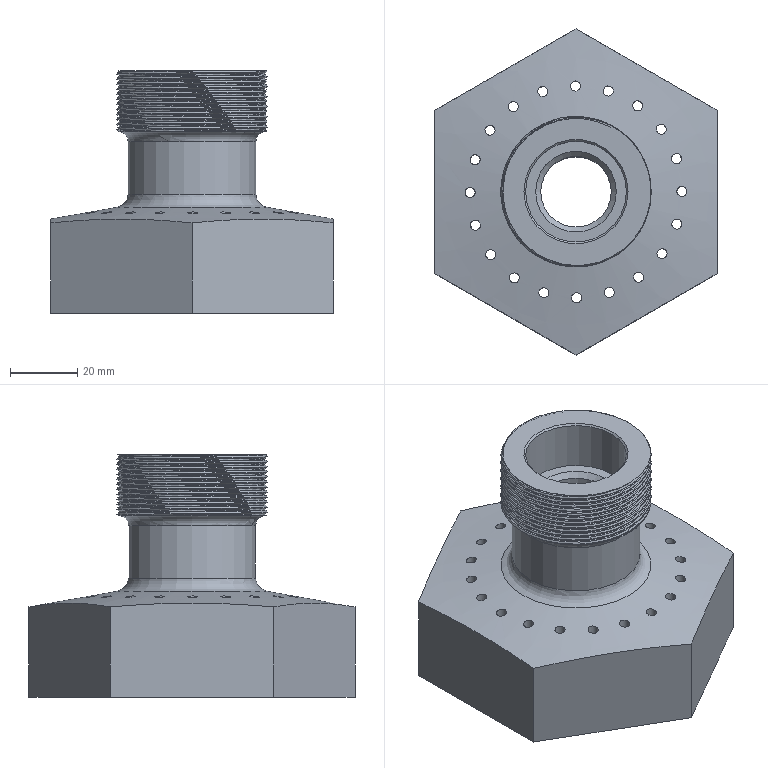Part | NX | features CYLINDER 5, DATUM_CSYS 5, SKETCH 4, BLEND 3, CHAMFER 2, EXTRUDE 2, HOLE PACKAGE 2, SIMPLE HOLE 2, SWP104 2, THREADS 2, REPLACE_FACE 1, SYMBOLIC_THREAD 1 | 1 solid | 56 faces | box 84 x 96.995 x 72 mm | volume 147613 mm3 | cylinder 29 | plane 14 | spline 6 | cone 4 | torus 3 | commonest cylinder face diameters 3 x20 72 x2 21 x1 30 x1 38 x1 40 x1